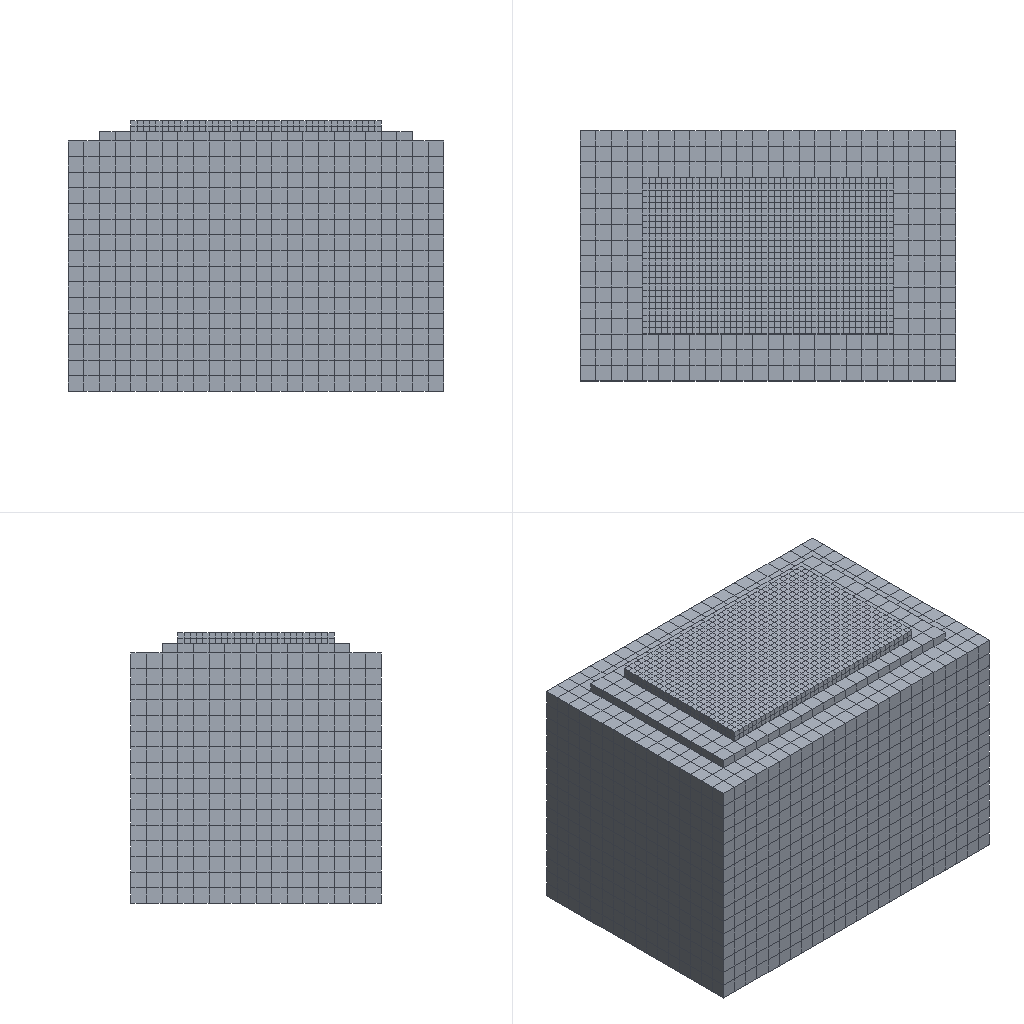Simulation study | abaqus
Set-up summary:
category,name,step,type,value,unit,region
solver,abaqus
solver,version,,,Abaqus/Standard 3DEXPERIENCE R2017x
units,not stated in the deck,,not stated
analysis,deck,,static,static
load_step,Step-1,Step-1,static
load_step,requested,,,1
mesh,nodes,,,10969
mesh,elements,,,8384
element_type,C3D8R,,solid,8384
load,load commands in deck,,count,1
bc,support commands in deck,,count,3
material,DAOMIAN,,in results
material,DIJI,,in results
material,JICENG,,in results
check,setup vs results,,match,"per instance, exact: element labels, types and connectivity; labels of the nodes the elements use; coordinates of those nodes at SINGLE_PRECISION in 1 of 3 instance(s)"
Abaqus input file, long lists of numbers shortened:
*Heading
** Job name: Job-1 Model name: Model-1
** Generated by: Abaqus/CAE 2017
*Preprint, echo=NO, model=NO, history=NO, contact=NO
**
** PARTS
**
*Part, name=crack
*End Part
**
*Part, name=daomian
*Node
      1,           0.,          -5.,  0.35
      2,           0.,  -4.8,  0.35
** (3196 more lines like these left out)
*Element, type=C3D8R
   1,   79,   80,  106,  105,    1,    2,   28,   27
   2,   80,   81,  107,  106,    2,    3,   29,   28
** (1998 more lines like these left out)
*Nset, nset=Set-1, generate
    1,  3198,     1
*Elset, elset=Set-1, generate
    1,  2000,     1
** Section: daomian
*Solid Section, elset=Set-1, material=daomian
,
*End Part
**
*Part, name=diji
*Node
      1,           0.,          -8.,           8.
      2,           0.,         -7.5,           8.
** (7223 more lines like these left out)
*Element, type=C3D8R
   1,  290,  291,  308,  307,    1,    2,   19,   18
   2,  291,  292,  309,  308,    2,    3,   20,   19
** (6142 more lines like these left out)
*Nset, nset=Set-1, generate
    1,  7225,     1
*Elset, elset=Set-1, generate
    1,  6144,     1
** Section: diji
*Solid Section, elset=Set-1, material=diji
,
*End Part
**
*Part, name=jiceng
*Node
      1,           0.,          -6.,  0.3
      2,           0.,         -5.5,  0.3
** (544 more lines like these left out)
*Element, type=C3D8R
  1,  27,  28,  41,  40,   1,   2,  15,  14
  2,  28,  29,  42,  41,   2,   3,  16,  15
** (238 more lines like these left out)
*Nset, nset=Set-1, generate
   1,  546,    1
*Elset, elset=Set-1, generate
   1,  240,    1
** Section: jiceng
*Solid Section, elset=Set-1, material=jiceng
,
*End Part
**
**
** ASSEMBLY
**
*Assembly, name=Assembly
**
*Instance, name=daomian-1, part=daomian
          0.,          2.5,        -0.35
*End Instance
**
*Instance, name=jiceng-1, part=jiceng
         -1.,           3.,        -0.65
*End Instance
**
*Instance, name=diji-1, part=diji
         -2.,           4.,        -8.65
*End Instance
**
*Instance, name=crack-1, part=crack
          4.,           2.,         -0.1
          4.,           2.,         -0.1, 3.423, 1.423, 0.4774, 120.
*End Instance
**
*Nset, nset=Set-3, instance=diji-1
  273,  274,  275,  276,  277,  278,  279,  280,  281,  282,  283,  284,  285,  286,  287,  288
  289,  562,  563,  564,  565,  566,  567,  568,  569,  570,  571,  572,  573,  574,  575,  576
** (25 more lines like these left out)
*Elset, elset=Set-3, instance=diji-1
  241,  242,  243,  244,  245,  246,  247,  248,  249,  250,  251,  252,  253,  254,  255,  256
  497,  498,  499,  500,  501,  502,  503,  504,  505,  506,  507,  508,  509,  510,  511,  512
** (22 more lines like these left out)
*Nset, nset=Set-4, instance=diji-1
    1,    2,    3,    4,    5,    6,    7,    8,    9,   10,   11,   12,   13,   14,   15,   16
   17,   18,   19,   20,   21,   22,   23,   24,   25,   26,   27,   28,   29,   30,   31,   32
** (35 more lines like these left out)
*Elset, elset=Set-4, instance=diji-1
    1,    2,    3,    4,    5,    6,    7,    8,    9,   10,   11,   12,   13,   14,   15,   16
   17,   18,   19,   20,   21,   22,   23,   24,   25,   26,   27,   28,   29,   30,   31,   32
** (30 more lines like these left out)
*Nset, nset=Set-5, instance=diji-1
    1,   17,   18,   34,   35,   51,   52,   68,   69,   85,   86,  102,  103,  119,  120,  136
  137,  153,  154,  170,  171,  187,  188,  204,  205,  221,  222,  238,  239,  255,  256,  272
** (52 more lines like these left out)
*Elset, elset=Set-5, instance=diji-1
    1,   16,   17,   32,   33,   48,   49,   64,   65,   80,   81,   96,   97,  112,  113,  128
  129,  144,  145,  160,  161,  176,  177,  192,  193,  208,  209,  224,  225,  240,  241,  256
** (46 more lines like these left out)
*Nset, nset=_PickedSet10, internal, instance=daomian-1, generate
    1,  3198,     1
*Elset, elset=_PickedSet10, internal, instance=daomian-1, generate
    1,  2000,     1
*Elset, elset=_Surf-5_S3, internal, instance=daomian-1
    1,    2,    3,    4,    5,    6,    7,    8,    9,   10,   11,   12,   13,   14,   15,   16
   17,   18,   19,   20,   21,   22,   23,   24,   25,   51,   52,   53,   54,   55,   56,   57
** (61 more lines like these left out)
*Surface, type=ELEMENT, name=Surf-5
_Surf-5_S3, S3
*Elset, elset=_m_Surf-1_S3, internal, instance=jiceng-1, generate
   1,  240,    1
*Surface, type=ELEMENT, name=m_Surf-1
_m_Surf-1_S3, S3
*Elset, elset=_m_Surf-3_S5, internal, instance=jiceng-1, generate
   1,  240,    1
*Surface, type=ELEMENT, name=m_Surf-3
_m_Surf-3_S5, S5
*Elset, elset=_s_Surf-1_S5, internal, instance=daomian-1
   26,   27,   28,   29,   30,   31,   32,   33,   34,   35,   36,   37,   38,   39,   40,   41
   42,   43,   44,   45,   46,   47,   48,   49,   50,   76,   77,   78,   79,   80,   81,   82
** (61 more lines like these left out)
*Surface, type=ELEMENT, name=s_Surf-1
_s_Surf-1_S5, S5
*Elset, elset=_s_Surf-3_S3, internal, instance=diji-1
    1,    2,    3,    4,    5,    6,    7,    8,    9,   10,   11,   12,   13,   14,   15,   16
  257,  258,  259,  260,  261,  262,  263,  264,  265,  266,  267,  268,  269,  270,  271,  272
** (22 more lines like these left out)
*Surface, type=ELEMENT, name=s_Surf-3
_s_Surf-3_S3, S3
** Constraint: Constraint-1
*Tie, name=Constraint-1, adjust=yes
s_Surf-1, m_Surf-1
** Constraint: Constraint-2
*Tie, name=Constraint-2, adjust=yes
s_Surf-3, m_Surf-3
*Enrichment, name=Crack-1, type=PROPAGATION CRACK, elset=_PickedSet10
*End Assembly
**
** MATERIALS
**
*Material, name=daomian
*Damage Initiation, criterion=MAXPS
200000.,
*Damage Evolution, type=DISPLACEMENT
 1e-19,
*Damage Stabilization
0.001
*Density
2500.,
*Elastic
 3.8e+10, 0.15
*Material, name=diji
*Density
1800.,
*Elastic
 9e+07, 0.4
*Material, name=jiceng
*Density
2000.,
*Elastic
 1.5e+09, 0.25
*Initial Conditions, type=ENRICHMENT
daomian-1.102, 1,Crack-1, -0.2, 0.07071
daomian-1.102, 2,Crack-1, -0.2, -0.07071
daomian-1.102, 3,Crack-1, -0.2, 0.05303
daomian-1.102, 4,Crack-1, -0.2, 0.1945
daomian-1.102, 5,Crack-1, 1e-06, 0.07071
daomian-1.102, 6,Crack-1, 1e-06, -0.07071
daomian-1.102, 7,Crack-1, 1e-06, 0.05303
daomian-1.102, 8,Crack-1, 1e-06, 0.1945
daomian-1.102, 1,Crack-1, -0.2, -0.07071
daomian-1.102, 2,Crack-1, -0.2, -0.1
daomian-1.102, 3,Crack-1, -0.2, 0.075
daomian-1.102, 4,Crack-1, -0.2, 0.05303
daomian-1.102, 5,Crack-1, 1e-06, -0.07071
daomian-1.102, 6,Crack-1, 1e-06, -0.1
daomian-1.102, 7,Crack-1, 1e-06, 0.075
daomian-1.102, 8,Crack-1, 1e-06, 0.05303
daomian-1.103, 1,Crack-1, -0.2, -0.1
daomian-1.103, 2,Crack-1, -0.2, -0.1
daomian-1.103, 3,Crack-1, -0.2, 0.075
daomian-1.103, 4,Crack-1, -0.2, 0.075
daomian-1.103, 5,Crack-1, 1e-06, -0.1
daomian-1.103, 6,Crack-1, 1e-06, -0.1
daomian-1.103, 7,Crack-1, 1e-06, 0.075
daomian-1.103, 8,Crack-1, 1e-06, 0.075
** ----------------------------------------------------------------
**
** STEP: Step-1
**
*Step, name=Step-1, nlgeom=YES, inc=1000
*Static, stabilize=0.0002, allsdtol=0.05, continue=NO
0.01, 1., 1e-07, 0.1
**
** BOUNDARY CONDITIONS
**
** Name: [REDACTED] : Displacement/rotation angle
*Boundary
Set-3, 3, 3
** Name: x Type: Displacement/Rotation
*Boundary
Set-4, 1, 1
** Name: y Type: Displacement/Rotation
*Boundary
Set-5, 2, 2
**
** LOADS
**
** Name: Load-1   Type: Pressure
*Dsload
Surf-5, PNU, 1.
**
** CONTROLS
**
*Controls, reset
*Controls, parameters=time incrementation
, , , , , , , 15, , ,
**
** OUTPUT REQUESTS
**
*Restart, write, frequency=0
**
** FIELD OUTPUT: F-Output-1
**
*Output, field
*Node Output
CF, PHILSM, PSILSM, RF, RM, RT, TF, U
V
*Element Output, directions=YES
DMICRT, E, LE, MISES, MISESMAX, MISESONLY, NE, PE, PEEQ, PEEQMAX, PEEQT, PEMAG, PRESSONLY, S, SDEG, SDV
SF, SSAVG, STATUSXFEM
*Contact Output
CDISP, CSTRESS
**
** HISTORY OUTPUT: H-Output-1
**
*Output, history, variable=PRESELECT
*End Step
Results summary:
result,step,,completed,increments=96 time=1.0/1.0
result,analysis,,,static
result,last_loadstep,,,1
result,primary field,,,U
result,reaction total,,FX,147.335,model units
result,reaction total,,FY,0.1557,model units
result,reaction total,,FZ,267223.37,model units